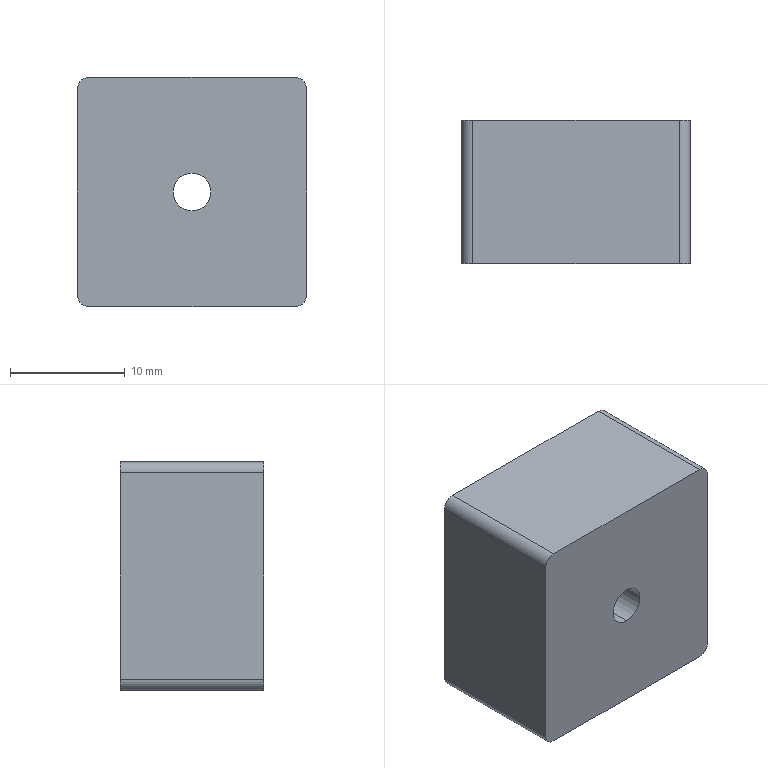Part | SolidWorks | features Extrusion 1, Fillet 1, HoleWzd 1 | 1 solid | 12 faces | box 20 x 12.5 x 20 mm | volume 4882 mm3 | cylinder 6 | plane 6 | commonest cylinder face diameters 2 x4 3.3 x2
STEP:
#1=CARTESIAN_POINT('',(0.,0.,-1.65));
#2=VERTEX_POINT('',#1);
#3=CARTESIAN_POINT('',(0.,0.,1.65));
#4=VERTEX_POINT('',#3);
#5=CARTESIAN_POINT('',(0.,0.,0.));
#6=DIRECTION('',(0.,1.,0.));
#7=DIRECTION('',(0.,0.,1.));
#8=AXIS2_PLACEMENT_3D('',#5,#6,#7);
#9=CIRCLE('',#8,1.65);
#10=EDGE_CURVE('',#2,#4,#9,.T.);
#11=ORIENTED_EDGE('',*,*,#10,.F.);
#12=CARTESIAN_POINT('',(0.,12.5,-1.65));
#13=VERTEX_POINT('',#12);
#14=CARTESIAN_POINT('',(0.,12.5,-1.65));
#15=DIRECTION('',(0.,1.,0.));
#16=VECTOR('',#15,1000.);
#17=LINE('',#14,#16);
#18=EDGE_CURVE('',#2,#13,#17,.T.);
#19=ORIENTED_EDGE('',*,*,#18,.T.);
#20=CARTESIAN_POINT('',(0.,12.5,1.65));
#21=VERTEX_POINT('',#20);
#22=CARTESIAN_POINT('',(0.,12.5,0.));
#23=DIRECTION('',(0.,1.,0.));
#24=DIRECTION('',(0.,0.,1.));
#25=AXIS2_PLACEMENT_3D('',#22,#23,#24);
#26=CIRCLE('',#25,1.65);
#27=EDGE_CURVE('',#13,#21,#26,.T.);
#28=ORIENTED_EDGE('',*,*,#27,.T.);
#29=CARTESIAN_POINT('',(0.,12.5,1.65));
#30=DIRECTION('',(0.,1.,0.));
#31=VECTOR('',#30,1000.);
#32=LINE('',#29,#31);
#33=EDGE_CURVE('',#4,#21,#32,.T.);
#34=ORIENTED_EDGE('',*,*,#33,.F.);
#35=EDGE_LOOP('',(#11,#19,#28,#34));
#36=FACE_OUTER_BOUND('',#35,.T.);
#37=CARTESIAN_POINT('',(0.,12.5,0.));
#38=DIRECTION('',(0.,1.,0.));
#39=DIRECTION('',(0.,0.,1.));
#40=AXIS2_PLACEMENT_3D('',#37,#38,#39);
#41=CYLINDRICAL_SURFACE('',#40,1.65);
#42=ADVANCED_FACE('',(#36),#41,.F.);
#43=CARTESIAN_POINT('',(10.,0.,9.));
#44=VERTEX_POINT('',#43);
#45=CARTESIAN_POINT('',(10.,0.,-9.));
#46=VERTEX_POINT('',#45);
#47=CARTESIAN_POINT('',(10.,0.,-10.));
#48=DIRECTION('',(0.,0.,-1.));
#49=VECTOR('',#48,1000.);
#50=LINE('',#47,#49);
#51=EDGE_CURVE('',#44,#46,#50,.T.);
#52=ORIENTED_EDGE('',*,*,#51,.T.);
#53=CARTESIAN_POINT('',(10.,12.5,-9.));
#54=VERTEX_POINT('',#53);
#55=CARTESIAN_POINT('',(10.,12.5,-9.));
#56=DIRECTION('',(0.,1.,0.));
#57=VECTOR('',#56,1000.);
#58=LINE('',#55,#57);
#59=EDGE_CURVE('',#46,#54,#58,.T.);
#60=ORIENTED_EDGE('',*,*,#59,.T.);
#61=CARTESIAN_POINT('',(10.,12.5,9.));
#62=VERTEX_POINT('',#61);
#63=CARTESIAN_POINT('',(10.,12.5,-10.));
#64=DIRECTION('',(0.,0.,-1.));
#65=VECTOR('',#64,1000.);
#66=LINE('',#63,#65);
#67=EDGE_CURVE('',#62,#54,#66,.T.);
#68=ORIENTED_EDGE('',*,*,#67,.F.);
#69=CARTESIAN_POINT('',(10.,12.5,9.));
#70=DIRECTION('',(0.,-1.,0.));
#71=VECTOR('',#70,1000.);
#72=LINE('',#69,#71);
#73=EDGE_CURVE('',#62,#44,#72,.T.);
#74=ORIENTED_EDGE('',*,*,#73,.T.);
#75=EDGE_LOOP('',(#52,#60,#68,#74));
#76=FACE_OUTER_BOUND('',#75,.T.);
#77=CARTESIAN_POINT('',(10.,12.5,-10.));
#78=DIRECTION('',(-1.,0.,0.));
#79=DIRECTION('',(0.,0.,1.));
#80=AXIS2_PLACEMENT_3D('',#77,#78,#79);
#81=PLANE('',#80);
#82=ADVANCED_FACE('',(#76),#81,.F.);
#83=CARTESIAN_POINT('',(9.,0.,-10.));
#84=VERTEX_POINT('',#83);
#85=CARTESIAN_POINT('',(-9.,0.,-10.));
#86=VERTEX_POINT('',#85);
#87=CARTESIAN_POINT('',(-10.,0.,-10.));
#88=DIRECTION('',(-1.,0.,0.));
#89=VECTOR('',#88,1000.);
#90=LINE('',#87,#89);
#91=EDGE_CURVE('',#84,#86,#90,.T.);
#92=ORIENTED_EDGE('',*,*,#91,.T.);
#93=CARTESIAN_POINT('',(-9.,12.5,-10.));
#94=VERTEX_POINT('',#93);
#95=CARTESIAN_POINT('',(-9.,12.5,-10.));
#96=DIRECTION('',(0.,1.,0.));
#97=VECTOR('',#96,1000.);
#98=LINE('',#95,#97);
#99=EDGE_CURVE('',#86,#94,#98,.T.);
#100=ORIENTED_EDGE('',*,*,#99,.T.);
#101=CARTESIAN_POINT('',(9.,12.5,-10.));
#102=VERTEX_POINT('',#101);
#103=CARTESIAN_POINT('',(-10.,12.5,-10.));
#104=DIRECTION('',(-1.,0.,0.));
#105=VECTOR('',#104,1000.);
#106=LINE('',#103,#105);
#107=EDGE_CURVE('',#102,#94,#106,.T.);
#108=ORIENTED_EDGE('',*,*,#107,.F.);
#109=CARTESIAN_POINT('',(9.,12.5,-10.));
#110=DIRECTION('',(0.,-1.,0.));
#111=VECTOR('',#110,1000.);
#112=LINE('',#109,#111);
#113=EDGE_CURVE('',#102,#84,#112,.T.);
#114=ORIENTED_EDGE('',*,*,#113,.T.);
#115=EDGE_LOOP('',(#92,#100,#108,#114));
#116=FACE_OUTER_BOUND('',#115,.T.);
#117=CARTESIAN_POINT('',(-10.,12.5,-10.));
#118=DIRECTION('',(0.,0.,1.));
#119=DIRECTION('',(1.,0.,0.));
#120=AXIS2_PLACEMENT_3D('',#117,#118,#119);
#121=PLANE('',#120);
#122=ADVANCED_FACE('',(#116),#121,.F.);
#123=CARTESIAN_POINT('',(-10.,12.5,-9.));
#124=VERTEX_POINT('',#123);
#125=CARTESIAN_POINT('',(-10.,12.5,9.));
#126=VERTEX_POINT('',#125);
#127=CARTESIAN_POINT('',(-10.,12.5,-10.));
#128=DIRECTION('',(0.,0.,1.));
#129=VECTOR('',#128,1000.);
#130=LINE('',#127,#129);
#131=EDGE_CURVE('',#124,#126,#130,.T.);
#132=ORIENTED_EDGE('',*,*,#131,.F.);
#133=CARTESIAN_POINT('',(-10.,0.,-9.));
#134=VERTEX_POINT('',#133);
#135=CARTESIAN_POINT('',(-10.,12.5,-9.));
#136=DIRECTION('',(0.,-1.,0.));
#137=VECTOR('',#136,1000.);
#138=LINE('',#135,#137);
#139=EDGE_CURVE('',#124,#134,#138,.T.);
#140=ORIENTED_EDGE('',*,*,#139,.T.);
#141=CARTESIAN_POINT('',(-10.,0.,9.));
#142=VERTEX_POINT('',#141);
#143=CARTESIAN_POINT('',(-10.,0.,-10.));
#144=DIRECTION('',(0.,0.,1.));
#145=VECTOR('',#144,1000.);
#146=LINE('',#143,#145);
#147=EDGE_CURVE('',#134,#142,#146,.T.);
#148=ORIENTED_EDGE('',*,*,#147,.T.);
#149=CARTESIAN_POINT('',(-10.,12.5,9.));
#150=DIRECTION('',(0.,1.,0.));
#151=VECTOR('',#150,1000.);
#152=LINE('',#149,#151);
#153=EDGE_CURVE('',#142,#126,#152,.T.);
#154=ORIENTED_EDGE('',*,*,#153,.T.);
#155=EDGE_LOOP('',(#132,#140,#148,#154));
#156=FACE_OUTER_BOUND('',#155,.T.);
#157=CARTESIAN_POINT('',(-10.,12.5,-10.));
#158=DIRECTION('',(1.,0.,0.));
#159=DIRECTION('',(0.,0.,-1.));
#160=AXIS2_PLACEMENT_3D('',#157,#158,#159);
#161=PLANE('',#160);
#162=ADVANCED_FACE('',(#156),#161,.F.);
#163=CARTESIAN_POINT('',(-9.,0.,10.));
#164=VERTEX_POINT('',#163);
#165=CARTESIAN_POINT('',(9.,0.,10.));
#166=VERTEX_POINT('',#165);
#167=CARTESIAN_POINT('',(-10.,0.,10.));
#168=DIRECTION('',(1.,0.,0.));
#169=VECTOR('',#168,1000.);
#170=LINE('',#167,#169);
#171=EDGE_CURVE('',#164,#166,#170,.T.);
#172=ORIENTED_EDGE('',*,*,#171,.T.);
#173=CARTESIAN_POINT('',(9.,12.5,10.));
#174=VERTEX_POINT('',#173);
#175=CARTESIAN_POINT('',(9.,12.5,10.));
#176=DIRECTION('',(0.,1.,0.));
#177=VECTOR('',#176,1000.);
#178=LINE('',#175,#177);
#179=EDGE_CURVE('',#166,#174,#178,.T.);
#180=ORIENTED_EDGE('',*,*,#179,.T.);
#181=CARTESIAN_POINT('',(-9.,12.5,10.));
#182=VERTEX_POINT('',#181);
#183=CARTESIAN_POINT('',(-10.,12.5,10.));
#184=DIRECTION('',(1.,0.,0.));
#185=VECTOR('',#184,1000.);
#186=LINE('',#183,#185);
#187=EDGE_CURVE('',#182,#174,#186,.T.);
#188=ORIENTED_EDGE('',*,*,#187,.F.);
#189=CARTESIAN_POINT('',(-9.,12.5,10.));
#190=DIRECTION('',(0.,-1.,0.));
#191=VECTOR('',#190,1000.);
#192=LINE('',#189,#191);
#193=EDGE_CURVE('',#182,#164,#192,.T.);
#194=ORIENTED_EDGE('',*,*,#193,.T.);
#195=EDGE_LOOP('',(#172,#180,#188,#194));
#196=FACE_OUTER_BOUND('',#195,.T.);
#197=CARTESIAN_POINT('',(-10.,12.5,10.));
#198=DIRECTION('',(0.,0.,-1.));
#199=DIRECTION('',(-1.,0.,0.));
#200=AXIS2_PLACEMENT_3D('',#197,#198,#199);
#201=PLANE('',#200);
#202=ADVANCED_FACE('',(#196),#201,.F.);
#203=CARTESIAN_POINT('',(0.,12.5,0.));
#204=DIRECTION('',(0.,1.,0.));
#205=DIRECTION('',(0.,0.,1.));
#206=AXIS2_PLACEMENT_3D('',#203,#204,#205);
#207=CIRCLE('',#206,1.65);
#208=EDGE_CURVE('',#21,#13,#207,.T.);
#209=ORIENTED_EDGE('',*,*,#208,.F.);
#210=ORIENTED_EDGE('',*,*,#27,.F.);
#211=EDGE_LOOP('',(#209,#210));
#212=FACE_BOUND('',#211,.T.);
#213=ORIENTED_EDGE('',*,*,#107,.T.);
#214=CARTESIAN_POINT('',(-9.,12.5,-9.));
#215=DIRECTION('',(0.,1.,0.));
#216=DIRECTION('',(0.,0.,1.));
#217=AXIS2_PLACEMENT_3D('',#214,#215,#216);
#218=CIRCLE('',#217,1.);
#219=EDGE_CURVE('',#94,#124,#218,.T.);
#220=ORIENTED_EDGE('',*,*,#219,.T.);
#221=ORIENTED_EDGE('',*,*,#131,.T.);
#222=CARTESIAN_POINT('',(-9.,12.5,9.));
#223=DIRECTION('',(0.,1.,0.));
#224=DIRECTION('',(0.,0.,1.));
#225=AXIS2_PLACEMENT_3D('',#222,#223,#224);
#226=CIRCLE('',#225,1.);
#227=EDGE_CURVE('',#126,#182,#226,.T.);
#228=ORIENTED_EDGE('',*,*,#227,.T.);
#229=ORIENTED_EDGE('',*,*,#187,.T.);
#230=CARTESIAN_POINT('',(9.,12.5,9.));
#231=DIRECTION('',(0.,1.,0.));
#232=DIRECTION('',(0.,0.,1.));
#233=AXIS2_PLACEMENT_3D('',#230,#231,#232);
#234=CIRCLE('',#233,1.);
#235=EDGE_CURVE('',#174,#62,#234,.T.);
#236=ORIENTED_EDGE('',*,*,#235,.T.);
#237=ORIENTED_EDGE('',*,*,#67,.T.);
#238=CARTESIAN_POINT('',(9.,12.5,-9.));
#239=DIRECTION('',(0.,1.,0.));
#240=DIRECTION('',(0.,0.,1.));
#241=AXIS2_PLACEMENT_3D('',#238,#239,#240);
#242=CIRCLE('',#241,1.);
#243=EDGE_CURVE('',#54,#102,#242,.T.);
#244=ORIENTED_EDGE('',*,*,#243,.T.);
#245=EDGE_LOOP('',(#213,#220,#221,#228,#229,#236,#237,#244));
#246=FACE_OUTER_BOUND('',#245,.T.);
#247=CARTESIAN_POINT('',(0.,12.5,0.));
#248=DIRECTION('',(0.,1.,0.));
#249=DIRECTION('',(0.,0.,1.));
#250=AXIS2_PLACEMENT_3D('',#247,#248,#249);
#251=PLANE('',#250);
#252=ADVANCED_FACE('',(#212,#246),#251,.T.);
#253=CARTESIAN_POINT('',(0.,0.,0.));
#254=DIRECTION('',(0.,1.,0.));
#255=DIRECTION('',(0.,0.,1.));
#256=AXIS2_PLACEMENT_3D('',#253,#254,#255);
#257=CIRCLE('',#256,1.65);
#258=EDGE_CURVE('',#4,#2,#257,.T.);
#259=ORIENTED_EDGE('',*,*,#258,.T.);
#260=ORIENTED_EDGE('',*,*,#10,.T.);
#261=EDGE_LOOP('',(#259,#260));
#262=FACE_BOUND('',#261,.T.);
#263=ORIENTED_EDGE('',*,*,#147,.F.);
#264=CARTESIAN_POINT('',(-9.,0.,-9.));
#265=DIRECTION('',(0.,-1.,0.));
#266=DIRECTION('',(0.,0.,1.));
#267=AXIS2_PLACEMENT_3D('',#264,#265,#266);
#268=CIRCLE('',#267,1.);
#269=EDGE_CURVE('',#134,#86,#268,.T.);
#270=ORIENTED_EDGE('',*,*,#269,.T.);
#271=ORIENTED_EDGE('',*,*,#91,.F.);
#272=CARTESIAN_POINT('',(9.,0.,-9.));
#273=DIRECTION('',(0.,-1.,0.));
#274=DIRECTION('',(0.,0.,1.));
#275=AXIS2_PLACEMENT_3D('',#272,#273,#274);
#276=CIRCLE('',#275,1.);
#277=EDGE_CURVE('',#84,#46,#276,.T.);
#278=ORIENTED_EDGE('',*,*,#277,.T.);
#279=ORIENTED_EDGE('',*,*,#51,.F.);
#280=CARTESIAN_POINT('',(9.,0.,9.));
#281=DIRECTION('',(0.,-1.,0.));
#282=DIRECTION('',(0.,0.,1.));
#283=AXIS2_PLACEMENT_3D('',#280,#281,#282);
#284=CIRCLE('',#283,1.);
#285=EDGE_CURVE('',#44,#166,#284,.T.);
#286=ORIENTED_EDGE('',*,*,#285,.T.);
#287=ORIENTED_EDGE('',*,*,#171,.F.);
#288=CARTESIAN_POINT('',(-9.,0.,9.));
#289=DIRECTION('',(0.,-1.,0.));
#290=DIRECTION('',(0.,0.,1.));
#291=AXIS2_PLACEMENT_3D('',#288,#289,#290);
#292=CIRCLE('',#291,1.);
#293=EDGE_CURVE('',#164,#142,#292,.T.);
#294=ORIENTED_EDGE('',*,*,#293,.T.);
#295=EDGE_LOOP('',(#263,#270,#271,#278,#279,#286,#287,#294));
#296=FACE_OUTER_BOUND('',#295,.T.);
#297=CARTESIAN_POINT('',(0.,0.,0.));
#298=DIRECTION('',(0.,1.,0.));
#299=DIRECTION('',(0.,0.,1.));
#300=AXIS2_PLACEMENT_3D('',#297,#298,#299);
#301=PLANE('',#300);
#302=ADVANCED_FACE('',(#262,#296),#301,.F.);
#303=ORIENTED_EDGE('',*,*,#18,.F.);
#304=ORIENTED_EDGE('',*,*,#258,.F.);
#305=ORIENTED_EDGE('',*,*,#33,.T.);
#306=ORIENTED_EDGE('',*,*,#208,.T.);
#307=EDGE_LOOP('',(#303,#304,#305,#306));
#308=FACE_OUTER_BOUND('',#307,.T.);
#309=CARTESIAN_POINT('',(0.,12.5,0.));
#310=DIRECTION('',(0.,1.,0.));
#311=DIRECTION('',(0.,0.,1.));
#312=AXIS2_PLACEMENT_3D('',#309,#310,#311);
#313=CYLINDRICAL_SURFACE('',#312,1.65);
#314=ADVANCED_FACE('',(#308),#313,.F.);
#315=ORIENTED_EDGE('',*,*,#219,.F.);
#316=ORIENTED_EDGE('',*,*,#99,.F.);
#317=ORIENTED_EDGE('',*,*,#269,.F.);
#318=ORIENTED_EDGE('',*,*,#139,.F.);
#319=EDGE_LOOP('',(#315,#316,#317,#318));
#320=FACE_OUTER_BOUND('',#319,.T.);
#321=CARTESIAN_POINT('',(-9.,12.5,-9.));
#322=DIRECTION('',(0.,-1.,0.));
#323=DIRECTION('',(0.,0.,-1.));
#324=AXIS2_PLACEMENT_3D('',#321,#322,#323);
#325=CYLINDRICAL_SURFACE('',#324,1.);
#326=ADVANCED_FACE('',(#320),#325,.T.);
#327=ORIENTED_EDGE('',*,*,#243,.F.);
#328=ORIENTED_EDGE('',*,*,#59,.F.);
#329=ORIENTED_EDGE('',*,*,#277,.F.);
#330=ORIENTED_EDGE('',*,*,#113,.F.);
#331=EDGE_LOOP('',(#327,#328,#329,#330));
#332=FACE_OUTER_BOUND('',#331,.T.);
#333=CARTESIAN_POINT('',(9.,12.5,-9.));
#334=DIRECTION('',(0.,-1.,0.));
#335=DIRECTION('',(0.,0.,-1.));
#336=AXIS2_PLACEMENT_3D('',#333,#334,#335);
#337=CYLINDRICAL_SURFACE('',#336,1.);
#338=ADVANCED_FACE('',(#332),#337,.T.);
#339=ORIENTED_EDGE('',*,*,#235,.F.);
#340=ORIENTED_EDGE('',*,*,#179,.F.);
#341=ORIENTED_EDGE('',*,*,#285,.F.);
#342=ORIENTED_EDGE('',*,*,#73,.F.);
#343=EDGE_LOOP('',(#339,#340,#341,#342));
#344=FACE_OUTER_BOUND('',#343,.T.);
#345=CARTESIAN_POINT('',(9.,12.5,9.));
#346=DIRECTION('',(0.,-1.,0.));
#347=DIRECTION('',(0.,0.,-1.));
#348=AXIS2_PLACEMENT_3D('',#345,#346,#347);
#349=CYLINDRICAL_SURFACE('',#348,1.);
#350=ADVANCED_FACE('',(#344),#349,.T.);
#351=ORIENTED_EDGE('',*,*,#227,.F.);
#352=ORIENTED_EDGE('',*,*,#153,.F.);
#353=ORIENTED_EDGE('',*,*,#293,.F.);
#354=ORIENTED_EDGE('',*,*,#193,.F.);
#355=EDGE_LOOP('',(#351,#352,#353,#354));
#356=FACE_OUTER_BOUND('',#355,.T.);
#357=CARTESIAN_POINT('',(-9.,12.5,9.));
#358=DIRECTION('',(0.,-1.,0.));
#359=DIRECTION('',(0.,0.,-1.));
#360=AXIS2_PLACEMENT_3D('',#357,#358,#359);
#361=CYLINDRICAL_SURFACE('',#360,1.);
#362=ADVANCED_FACE('',(#356),#361,.T.);
#363=CLOSED_SHELL('',(#42,#82,#122,#162,#202,#252,#302,#314,#326,#338,#350,#362));
#364=MANIFOLD_SOLID_BREP('',#363);
#365=CARTESIAN_POINT('',(0.,0.,0.));
#366=DIRECTION('',(0.,0.,1.));
#367=DIRECTION('',(1.,0.,0.));
#368=AXIS2_PLACEMENT_3D('',#365,#366,#367);
#369=(LENGTH_UNIT()NAMED_UNIT(*)SI_UNIT(.MILLI.,.METRE.));
#370=UNCERTAINTY_MEASURE_WITH_UNIT(LENGTH_MEASURE(0.00001),#369,'','');
#371=(NAMED_UNIT(*)PLANE_ANGLE_UNIT()SI_UNIT($,.RADIAN.));
#372=(NAMED_UNIT(*)SI_UNIT($,.STERADIAN.)SOLID_ANGLE_UNIT());
#373=(GEOMETRIC_REPRESENTATION_CONTEXT(3)GLOBAL_UNCERTAINTY_ASSIGNED_CONTEXT((#370))GLOBAL_UNIT_ASSIGNED_CONTEXT((#369,#371,#372))REPRESENTATION_CONTEXT('',''));
#374=ADVANCED_BREP_SHAPE_REPRESENTATION('',(#364,#368),#373);